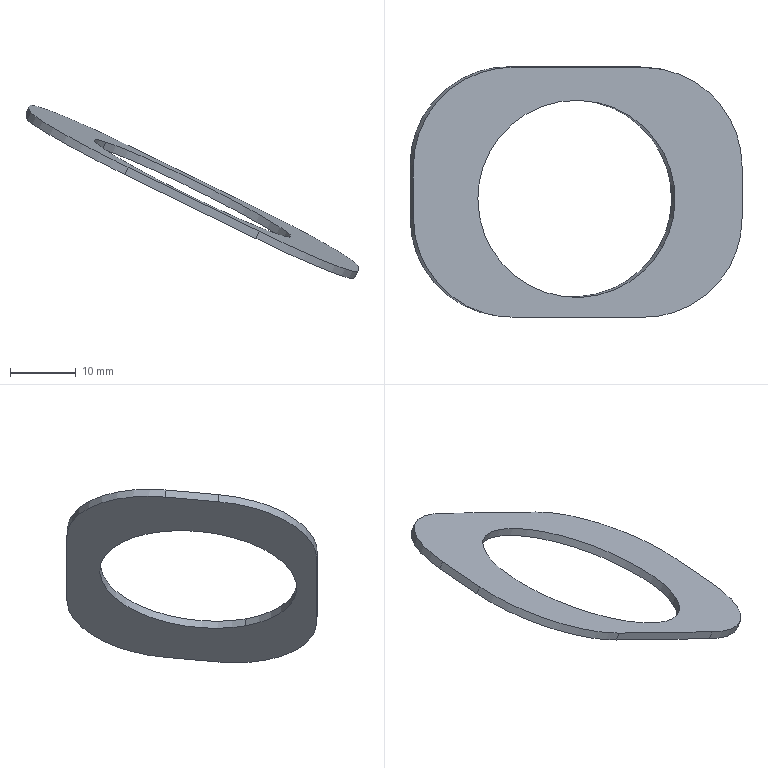Part | 1 solid | 12 faces | box 50.524 x 38.094 x 26.395 mm | volume 1339 mm3 | spline 12